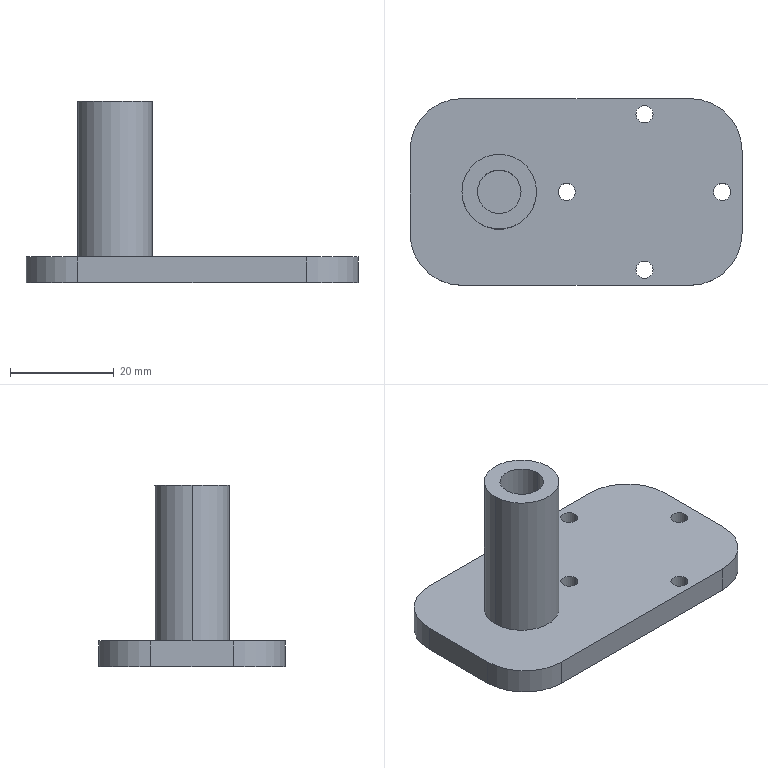Part | SolidWorks | features MirrorStock 1 | 1 solid | 24 faces | box 64 x 36 x 35 mm | volume 14420 mm3 | cylinder 16 | plane 8 | commonest cylinder face diameters 3.3 x8 20 x4 8.4 x2 14.4 x2
STEP:
#1=CARTESIAN_POINT('',(29.65,15.,-22.5));
#2=VERTEX_POINT('',#1);
#3=CARTESIAN_POINT('',(26.35,15.,-22.5));
#4=VERTEX_POINT('',#3);
#5=CARTESIAN_POINT('',(28.,15.,-22.5));
#6=DIRECTION('',(0.,0.,1.));
#7=DIRECTION('',(1.,0.,0.));
#8=AXIS2_PLACEMENT_3D('',#5,#6,#7);
#9=CIRCLE('',#8,1.65);
#10=EDGE_CURVE('',#2,#4,#9,.T.);
#11=ORIENTED_EDGE('',*,*,#10,.T.);
#12=CARTESIAN_POINT('',(26.35,15.,-27.5));
#13=VERTEX_POINT('',#12);
#14=CARTESIAN_POINT('',(26.35,15.,22.5));
#15=DIRECTION('',(0.,0.,-1.));
#16=VECTOR('',#15,1000.);
#17=LINE('',#14,#16);
#18=EDGE_CURVE('',#4,#13,#17,.T.);
#19=ORIENTED_EDGE('',*,*,#18,.T.);
#20=CARTESIAN_POINT('',(29.65,15.,-27.5));
#21=VERTEX_POINT('',#20);
#22=CARTESIAN_POINT('',(28.,15.,-27.5));
#23=DIRECTION('',(0.,0.,1.));
#24=DIRECTION('',(1.,0.,0.));
#25=AXIS2_PLACEMENT_3D('',#22,#23,#24);
#26=CIRCLE('',#25,1.65);
#27=EDGE_CURVE('',#21,#13,#26,.T.);
#28=ORIENTED_EDGE('',*,*,#27,.F.);
#29=CARTESIAN_POINT('',(29.65,15.,22.5));
#30=DIRECTION('',(0.,0.,-1.));
#31=VECTOR('',#30,1000.);
#32=LINE('',#29,#31);
#33=EDGE_CURVE('',#2,#21,#32,.T.);
#34=ORIENTED_EDGE('',*,*,#33,.F.);
#35=EDGE_LOOP('',(#11,#19,#28,#34));
#36=FACE_OUTER_BOUND('',#35,.T.);
#37=CARTESIAN_POINT('',(28.,15.,22.5));
#38=DIRECTION('',(0.,0.,-1.));
#39=DIRECTION('',(1.,0.,0.));
#40=AXIS2_PLACEMENT_3D('',#37,#38,#39);
#41=CYLINDRICAL_SURFACE('',#40,1.65);
#42=ADVANCED_FACE('',(#36),#41,.F.);
#43=CARTESIAN_POINT('',(44.65,0.,-22.5));
#44=VERTEX_POINT('',#43);
#45=CARTESIAN_POINT('',(41.35,0.,-22.5));
#46=VERTEX_POINT('',#45);
#47=CARTESIAN_POINT('',(43.,0.,-22.5));
#48=DIRECTION('',(0.,0.,1.));
#49=DIRECTION('',(1.,0.,0.));
#50=AXIS2_PLACEMENT_3D('',#47,#48,#49);
#51=CIRCLE('',#50,1.65);
#52=EDGE_CURVE('',#44,#46,#51,.T.);
#53=ORIENTED_EDGE('',*,*,#52,.T.);
#54=CARTESIAN_POINT('',(41.35,0.,-27.5));
#55=VERTEX_POINT('',#54);
#56=CARTESIAN_POINT('',(41.35,0.,22.5));
#57=DIRECTION('',(0.,0.,-1.));
#58=VECTOR('',#57,1000.);
#59=LINE('',#56,#58);
#60=EDGE_CURVE('',#46,#55,#59,.T.);
#61=ORIENTED_EDGE('',*,*,#60,.T.);
#62=CARTESIAN_POINT('',(44.65,0.,-27.5));
#63=VERTEX_POINT('',#62);
#64=CARTESIAN_POINT('',(43.,0.,-27.5));
#65=DIRECTION('',(0.,0.,1.));
#66=DIRECTION('',(1.,0.,0.));
#67=AXIS2_PLACEMENT_3D('',#64,#65,#66);
#68=CIRCLE('',#67,1.65);
#69=EDGE_CURVE('',#63,#55,#68,.T.);
#70=ORIENTED_EDGE('',*,*,#69,.F.);
#71=CARTESIAN_POINT('',(44.65,0.,22.5));
#72=DIRECTION('',(0.,0.,-1.));
#73=VECTOR('',#72,1000.);
#74=LINE('',#71,#73);
#75=EDGE_CURVE('',#44,#63,#74,.T.);
#76=ORIENTED_EDGE('',*,*,#75,.F.);
#77=EDGE_LOOP('',(#53,#61,#70,#76));
#78=FACE_OUTER_BOUND('',#77,.T.);
#79=CARTESIAN_POINT('',(43.,0.,22.5));
#80=DIRECTION('',(0.,0.,-1.));
#81=DIRECTION('',(1.,0.,0.));
#82=AXIS2_PLACEMENT_3D('',#79,#80,#81);
#83=CYLINDRICAL_SURFACE('',#82,1.65);
#84=ADVANCED_FACE('',(#78),#83,.F.);
#85=CARTESIAN_POINT('',(29.65,-15.,-22.5));
#86=VERTEX_POINT('',#85);
#87=CARTESIAN_POINT('',(26.35,-15.,-22.5));
#88=VERTEX_POINT('',#87);
#89=CARTESIAN_POINT('',(28.,-15.,-22.5));
#90=DIRECTION('',(0.,0.,1.));
#91=DIRECTION('',(1.,0.,0.));
#92=AXIS2_PLACEMENT_3D('',#89,#90,#91);
#93=CIRCLE('',#92,1.65);
#94=EDGE_CURVE('',#86,#88,#93,.T.);
#95=ORIENTED_EDGE('',*,*,#94,.T.);
#96=CARTESIAN_POINT('',(26.35,-15.,-27.5));
#97=VERTEX_POINT('',#96);
#98=CARTESIAN_POINT('',(26.35,-15.,22.5));
#99=DIRECTION('',(0.,0.,-1.));
#100=VECTOR('',#99,1000.);
#101=LINE('',#98,#100);
#102=EDGE_CURVE('',#88,#97,#101,.T.);
#103=ORIENTED_EDGE('',*,*,#102,.T.);
#104=CARTESIAN_POINT('',(29.65,-15.,-27.5));
#105=VERTEX_POINT('',#104);
#106=CARTESIAN_POINT('',(28.,-15.,-27.5));
#107=DIRECTION('',(0.,0.,1.));
#108=DIRECTION('',(1.,0.,0.));
#109=AXIS2_PLACEMENT_3D('',#106,#107,#108);
#110=CIRCLE('',#109,1.65);
#111=EDGE_CURVE('',#105,#97,#110,.T.);
#112=ORIENTED_EDGE('',*,*,#111,.F.);
#113=CARTESIAN_POINT('',(29.65,-15.,22.5));
#114=DIRECTION('',(0.,0.,-1.));
#115=VECTOR('',#114,1000.);
#116=LINE('',#113,#115);
#117=EDGE_CURVE('',#86,#105,#116,.T.);
#118=ORIENTED_EDGE('',*,*,#117,.F.);
#119=EDGE_LOOP('',(#95,#103,#112,#118));
#120=FACE_OUTER_BOUND('',#119,.T.);
#121=CARTESIAN_POINT('',(28.,-15.,22.5));
#122=DIRECTION('',(0.,0.,-1.));
#123=DIRECTION('',(1.,0.,0.));
#124=AXIS2_PLACEMENT_3D('',#121,#122,#123);
#125=CYLINDRICAL_SURFACE('',#124,1.65);
#126=ADVANCED_FACE('',(#120),#125,.F.);
#127=CARTESIAN_POINT('',(14.65,0.,-22.5));
#128=VERTEX_POINT('',#127);
#129=CARTESIAN_POINT('',(11.35,0.,-22.5));
#130=VERTEX_POINT('',#129);
#131=CARTESIAN_POINT('',(13.,0.,-22.5));
#132=DIRECTION('',(0.,0.,1.));
#133=DIRECTION('',(1.,0.,0.));
#134=AXIS2_PLACEMENT_3D('',#131,#132,#133);
#135=CIRCLE('',#134,1.65);
#136=EDGE_CURVE('',#128,#130,#135,.T.);
#137=ORIENTED_EDGE('',*,*,#136,.T.);
#138=CARTESIAN_POINT('',(11.35,0.,-27.5));
#139=VERTEX_POINT('',#138);
#140=CARTESIAN_POINT('',(11.35,0.,22.5));
#141=DIRECTION('',(0.,0.,-1.));
#142=VECTOR('',#141,1000.);
#143=LINE('',#140,#142);
#144=EDGE_CURVE('',#130,#139,#143,.T.);
#145=ORIENTED_EDGE('',*,*,#144,.T.);
#146=CARTESIAN_POINT('',(14.65,0.,-27.5));
#147=VERTEX_POINT('',#146);
#148=CARTESIAN_POINT('',(13.,0.,-27.5));
#149=DIRECTION('',(0.,0.,1.));
#150=DIRECTION('',(1.,0.,0.));
#151=AXIS2_PLACEMENT_3D('',#148,#149,#150);
#152=CIRCLE('',#151,1.65);
#153=EDGE_CURVE('',#147,#139,#152,.T.);
#154=ORIENTED_EDGE('',*,*,#153,.F.);
#155=CARTESIAN_POINT('',(14.65,0.,22.5));
#156=DIRECTION('',(0.,0.,-1.));
#157=VECTOR('',#156,1000.);
#158=LINE('',#155,#157);
#159=EDGE_CURVE('',#128,#147,#158,.T.);
#160=ORIENTED_EDGE('',*,*,#159,.F.);
#161=EDGE_LOOP('',(#137,#145,#154,#160));
#162=FACE_OUTER_BOUND('',#161,.T.);
#163=CARTESIAN_POINT('',(13.,0.,22.5));
#164=DIRECTION('',(0.,0.,-1.));
#165=DIRECTION('',(1.,0.,0.));
#166=AXIS2_PLACEMENT_3D('',#163,#164,#165);
#167=CYLINDRICAL_SURFACE('',#166,1.65);
#168=ADVANCED_FACE('',(#162),#167,.F.);
#169=CARTESIAN_POINT('',(-4.2,0.,-17.5));
#170=VERTEX_POINT('',#169);
#171=CARTESIAN_POINT('',(4.2,0.,-17.5));
#172=VERTEX_POINT('',#171);
#173=CARTESIAN_POINT('',(0.,0.,-17.5));
#174=DIRECTION('',(0.,0.,-1.));
#175=DIRECTION('',(-1.,0.,0.));
#176=AXIS2_PLACEMENT_3D('',#173,#174,#175);
#177=CIRCLE('',#176,4.2);
#178=EDGE_CURVE('',#170,#172,#177,.T.);
#179=ORIENTED_EDGE('',*,*,#178,.T.);
#180=CARTESIAN_POINT('',(4.2,0.,7.5));
#181=VERTEX_POINT('',#180);
#182=CARTESIAN_POINT('',(4.2,0.,-7.5));
#183=DIRECTION('',(0.,0.,1.));
#184=VECTOR('',#183,1000.);
#185=LINE('',#182,#184);
#186=EDGE_CURVE('',#172,#181,#185,.T.);
#187=ORIENTED_EDGE('',*,*,#186,.T.);
#188=CARTESIAN_POINT('',(-4.2,0.,7.5));
#189=VERTEX_POINT('',#188);
#190=CARTESIAN_POINT('',(0.,0.,7.5));
#191=DIRECTION('',(0.,0.,1.));
#192=DIRECTION('',(1.,0.,0.));
#193=AXIS2_PLACEMENT_3D('',#190,#191,#192);
#194=CIRCLE('',#193,4.2);
#195=EDGE_CURVE('',#181,#189,#194,.T.);
#196=ORIENTED_EDGE('',*,*,#195,.T.);
#197=CARTESIAN_POINT('',(-4.2,0.,-7.5));
#198=DIRECTION('',(0.,0.,1.));
#199=VECTOR('',#198,1000.);
#200=LINE('',#197,#199);
#201=EDGE_CURVE('',#170,#189,#200,.T.);
#202=ORIENTED_EDGE('',*,*,#201,.F.);
#203=EDGE_LOOP('',(#179,#187,#196,#202));
#204=FACE_OUTER_BOUND('',#203,.T.);
#205=CARTESIAN_POINT('',(0.,0.,-7.5));
#206=DIRECTION('',(0.,0.,1.));
#207=DIRECTION('',(-1.,0.,0.));
#208=AXIS2_PLACEMENT_3D('',#205,#206,#207);
#209=CYLINDRICAL_SURFACE('',#208,4.2);
#210=ADVANCED_FACE('',(#204),#209,.F.);
#211=CARTESIAN_POINT('',(-7.2,0.,-22.5));
#212=VERTEX_POINT('',#211);
#213=CARTESIAN_POINT('',(7.2,0.,-22.5));
#214=VERTEX_POINT('',#213);
#215=CARTESIAN_POINT('',(0.,0.,-22.5));
#216=DIRECTION('',(0.,0.,1.));
#217=DIRECTION('',(1.,0.,0.));
#218=AXIS2_PLACEMENT_3D('',#215,#216,#217);
#219=CIRCLE('',#218,7.2);
#220=EDGE_CURVE('',#212,#214,#219,.T.);
#221=ORIENTED_EDGE('',*,*,#220,.T.);
#222=CARTESIAN_POINT('',(7.2,0.,7.5));
#223=VERTEX_POINT('',#222);
#224=CARTESIAN_POINT('',(7.2,0.,-7.5));
#225=DIRECTION('',(0.,0.,1.));
#226=VECTOR('',#225,1000.);
#227=LINE('',#224,#226);
#228=EDGE_CURVE('',#214,#223,#227,.T.);
#229=ORIENTED_EDGE('',*,*,#228,.T.);
#230=CARTESIAN_POINT('',(-7.2,0.,7.5));
#231=VERTEX_POINT('',#230);
#232=CARTESIAN_POINT('',(0.,0.,7.5));
#233=DIRECTION('',(0.,0.,1.));
#234=DIRECTION('',(1.,0.,0.));
#235=AXIS2_PLACEMENT_3D('',#232,#233,#234);
#236=CIRCLE('',#235,7.2);
#237=EDGE_CURVE('',#231,#223,#236,.T.);
#238=ORIENTED_EDGE('',*,*,#237,.F.);
#239=CARTESIAN_POINT('',(-7.2,0.,-7.5));
#240=DIRECTION('',(0.,0.,1.));
#241=VECTOR('',#240,1000.);
#242=LINE('',#239,#241);
#243=EDGE_CURVE('',#212,#231,#242,.T.);
#244=ORIENTED_EDGE('',*,*,#243,.F.);
#245=EDGE_LOOP('',(#221,#229,#238,#244));
#246=FACE_OUTER_BOUND('',#245,.T.);
#247=CARTESIAN_POINT('',(0.,0.,-7.5));
#248=DIRECTION('',(0.,0.,1.));
#249=DIRECTION('',(-1.,0.,0.));
#250=AXIS2_PLACEMENT_3D('',#247,#248,#249);
#251=CYLINDRICAL_SURFACE('',#250,7.2);
#252=ADVANCED_FACE('',(#246),#251,.T.);
#253=ORIENTED_EDGE('',*,*,#228,.F.);
#254=CARTESIAN_POINT('',(0.,0.,-22.5));
#255=DIRECTION('',(0.,0.,1.));
#256=DIRECTION('',(1.,0.,0.));
#257=AXIS2_PLACEMENT_3D('',#254,#255,#256);
#258=CIRCLE('',#257,7.2);
#259=EDGE_CURVE('',#214,#212,#258,.T.);
#260=ORIENTED_EDGE('',*,*,#259,.T.);
#261=ORIENTED_EDGE('',*,*,#243,.T.);
#262=CARTESIAN_POINT('',(0.,0.,7.5));
#263=DIRECTION('',(0.,0.,1.));
#264=DIRECTION('',(1.,0.,0.));
#265=AXIS2_PLACEMENT_3D('',#262,#263,#264);
#266=CIRCLE('',#265,7.2);
#267=EDGE_CURVE('',#223,#231,#266,.T.);
#268=ORIENTED_EDGE('',*,*,#267,.F.);
#269=EDGE_LOOP('',(#253,#260,#261,#268));
#270=FACE_OUTER_BOUND('',#269,.T.);
#271=CARTESIAN_POINT('',(0.,0.,-7.5));
#272=DIRECTION('',(0.,0.,1.));
#273=DIRECTION('',(-1.,0.,0.));
#274=AXIS2_PLACEMENT_3D('',#271,#272,#273);
#275=CYLINDRICAL_SURFACE('',#274,7.2);
#276=ADVANCED_FACE('',(#270),#275,.T.);
#277=ORIENTED_EDGE('',*,*,#186,.F.);
#278=CARTESIAN_POINT('',(0.,0.,-17.5));
#279=DIRECTION('',(0.,0.,-1.));
#280=DIRECTION('',(-1.,0.,0.));
#281=AXIS2_PLACEMENT_3D('',#278,#279,#280);
#282=CIRCLE('',#281,4.2);
#283=EDGE_CURVE('',#172,#170,#282,.T.);
#284=ORIENTED_EDGE('',*,*,#283,.T.);
#285=ORIENTED_EDGE('',*,*,#201,.T.);
#286=CARTESIAN_POINT('',(0.,0.,7.5));
#287=DIRECTION('',(0.,0.,1.));
#288=DIRECTION('',(1.,0.,0.));
#289=AXIS2_PLACEMENT_3D('',#286,#287,#288);
#290=CIRCLE('',#289,4.2);
#291=EDGE_CURVE('',#189,#181,#290,.T.);
#292=ORIENTED_EDGE('',*,*,#291,.T.);
#293=EDGE_LOOP('',(#277,#284,#285,#292));
#294=FACE_OUTER_BOUND('',#293,.T.);
#295=CARTESIAN_POINT('',(0.,0.,-7.5));
#296=DIRECTION('',(0.,0.,1.));
#297=DIRECTION('',(-1.,0.,0.));
#298=AXIS2_PLACEMENT_3D('',#295,#296,#297);
#299=CYLINDRICAL_SURFACE('',#298,4.2);
#300=ADVANCED_FACE('',(#294),#299,.F.);
#301=ORIENTED_EDGE('',*,*,#291,.F.);
#302=ORIENTED_EDGE('',*,*,#195,.F.);
#303=EDGE_LOOP('',(#301,#302));
#304=FACE_BOUND('',#303,.T.);
#305=ORIENTED_EDGE('',*,*,#237,.T.);
#306=ORIENTED_EDGE('',*,*,#267,.T.);
#307=EDGE_LOOP('',(#305,#306));
#308=FACE_OUTER_BOUND('',#307,.T.);
#309=CARTESIAN_POINT('',(0.,0.,7.5));
#310=DIRECTION('',(0.,0.,-1.));
#311=DIRECTION('',(1.,0.,0.));
#312=AXIS2_PLACEMENT_3D('',#309,#310,#311);
#313=PLANE('',#312);
#314=ADVANCED_FACE('',(#304,#308),#313,.F.);
#315=CARTESIAN_POINT('',(-17.2,8.,-27.5));
#316=VERTEX_POINT('',#315);
#317=CARTESIAN_POINT('',(-17.2,-8.,-27.5));
#318=VERTEX_POINT('',#317);
#319=CARTESIAN_POINT('',(-17.2,-18.,-27.5));
#320=DIRECTION('',(0.,-1.,0.));
#321=VECTOR('',#320,1000.);
#322=LINE('',#319,#321);
#323=EDGE_CURVE('',#316,#318,#322,.T.);
#324=ORIENTED_EDGE('',*,*,#323,.T.);
#325=CARTESIAN_POINT('',(-17.2,-8.,-22.5));
#326=VERTEX_POINT('',#325);
#327=CARTESIAN_POINT('',(-17.2,-8.,-22.5));
#328=DIRECTION('',(0.,0.,-1.));
#329=VECTOR('',#328,1000.);
#330=LINE('',#327,#329);
#331=EDGE_CURVE('',#326,#318,#330,.T.);
#332=ORIENTED_EDGE('',*,*,#331,.F.);
#333=CARTESIAN_POINT('',(-17.2,8.,-22.5));
#334=VERTEX_POINT('',#333);
#335=CARTESIAN_POINT('',(-17.2,-18.,-22.5));
#336=DIRECTION('',(0.,-1.,0.));
#337=VECTOR('',#336,1000.);
#338=LINE('',#335,#337);
#339=EDGE_CURVE('',#334,#326,#338,.T.);
#340=ORIENTED_EDGE('',*,*,#339,.F.);
#341=CARTESIAN_POINT('',(-17.2,8.,-22.5));
#342=DIRECTION('',(0.,0.,1.));
#343=VECTOR('',#342,1000.);
#344=LINE('',#341,#343);
#345=EDGE_CURVE('',#316,#334,#344,.T.);
#346=ORIENTED_EDGE('',*,*,#345,.F.);
#347=EDGE_LOOP('',(#324,#332,#340,#346));
#348=FACE_OUTER_BOUND('',#347,.T.);
#349=CARTESIAN_POINT('',(-17.2,-18.,-22.5));
#350=DIRECTION('',(-1.,0.,0.));
#351=DIRECTION('',(0.,0.,-1.));
#352=AXIS2_PLACEMENT_3D('',#349,#350,#351);
#353=PLANE('',#352);
#354=ADVANCED_FACE('',(#348),#353,.T.);
#355=CARTESIAN_POINT('',(36.8,18.,-22.5));
#356=VERTEX_POINT('',#355);
#357=CARTESIAN_POINT('',(-7.2,18.,-22.5));
#358=VERTEX_POINT('',#357);
#359=CARTESIAN_POINT('',(46.8,18.,-22.5));
#360=DIRECTION('',(-1.,0.,0.));
#361=VECTOR('',#360,1000.);
#362=LINE('',#359,#361);
#363=EDGE_CURVE('',#356,#358,#362,.T.);
#364=ORIENTED_EDGE('',*,*,#363,.F.);
#365=CARTESIAN_POINT('',(36.8,18.,-27.5));
#366=VERTEX_POINT('',#365);
#367=CARTESIAN_POINT('',(36.8,18.,-22.5));
#368=DIRECTION('',(0.,0.,1.));
#369=VECTOR('',#368,1000.);
#370=LINE('',#367,#369);
#371=EDGE_CURVE('',#366,#356,#370,.T.);
#372=ORIENTED_EDGE('',*,*,#371,.F.);
#373=CARTESIAN_POINT('',(-7.2,18.,-27.5));
#374=VERTEX_POINT('',#373);
#375=CARTESIAN_POINT('',(46.8,18.,-27.5));
#376=DIRECTION('',(-1.,0.,0.));
#377=VECTOR('',#376,1000.);
#378=LINE('',#375,#377);
#379=EDGE_CURVE('',#366,#374,#378,.T.);
#380=ORIENTED_EDGE('',*,*,#379,.T.);
#381=CARTESIAN_POINT('',(-7.2,18.,-22.5));
#382=DIRECTION('',(0.,0.,-1.));
#383=VECTOR('',#382,1000.);
#384=LINE('',#381,#383);
#385=EDGE_CURVE('',#358,#374,#384,.T.);
#386=ORIENTED_EDGE('',*,*,#385,.F.);
#387=EDGE_LOOP('',(#364,#372,#380,#386));
#388=FACE_OUTER_BOUND('',#387,.T.);
#389=CARTESIAN_POINT('',(46.8,18.,-22.5));
#390=DIRECTION('',(0.,1.,0.));
#391=DIRECTION('',(-1.,0.,0.));
#392=AXIS2_PLACEMENT_3D('',#389,#390,#391);
#393=PLANE('',#392);
#394=ADVANCED_FACE('',(#388),#393,.T.);
#395=CARTESIAN_POINT('',(46.8,-8.,-27.5));
#396=VERTEX_POINT('',#395);
#397=CARTESIAN_POINT('',(46.8,8.,-27.5));
#398=VERTEX_POINT('',#397);
#399=CARTESIAN_POINT('',(46.8,-18.,-27.5));
#400=DIRECTION('',(0.,1.,0.));
#401=VECTOR('',#400,1000.);
#402=LINE('',#399,#401);
#403=EDGE_CURVE('',#396,#398,#402,.T.);
#404=ORIENTED_EDGE('',*,*,#403,.T.);
#405=CARTESIAN_POINT('',(46.8,8.,-22.5));
#406=VERTEX_POINT('',#405);
#407=CARTESIAN_POINT('',(46.8,8.,-22.5));
#408=DIRECTION('',(0.,0.,-1.));
#409=VECTOR('',#408,1000.);
#410=LINE('',#407,#409);
#411=EDGE_CURVE('',#406,#398,#410,.T.);
#412=ORIENTED_EDGE('',*,*,#411,.F.);
#413=CARTESIAN_POINT('',(46.8,-8.,-22.5));
#414=VERTEX_POINT('',#413);
#415=CARTESIAN_POINT('',(46.8,-18.,-22.5));
#416=DIRECTION('',(0.,1.,0.));
#417=VECTOR('',#416,1000.);
#418=LINE('',#415,#417);
#419=EDGE_CURVE('',#414,#406,#418,.T.);
#420=ORIENTED_EDGE('',*,*,#419,.F.);
#421=CARTESIAN_POINT('',(46.8,-8.,-22.5));
#422=DIRECTION('',(0.,0.,1.));
#423=VECTOR('',#422,1000.);
#424=LINE('',#421,#423);
#425=EDGE_CURVE('',#396,#414,#424,.T.);
#426=ORIENTED_EDGE('',*,*,#425,.F.);
#427=EDGE_LOOP('',(#404,#412,#420,#426));
#428=FACE_OUTER_BOUND('',#427,.T.);
#429=CARTESIAN_POINT('',(46.8,-18.,-22.5));
#430=DIRECTION('',(1.,0.,0.));
#431=DIRECTION('',(0.,0.,1.));
#432=AXIS2_PLACEMENT_3D('',#429,#430,#431);
#433=PLANE('',#432);
#434=ADVANCED_FACE('',(#428),#433,.T.);
#435=CARTESIAN_POINT('',(-7.2,-18.,-27.5));
#436=VERTEX_POINT('',#435);
#437=CARTESIAN_POINT('',(36.8,-18.,-27.5));
#438=VERTEX_POINT('',#437);
#439=CARTESIAN_POINT('',(46.8,-18.,-27.5));
#440=DIRECTION('',(1.,0.,0.));
#441=VECTOR('',#440,1000.);
#442=LINE('',#439,#441);
#443=EDGE_CURVE('',#436,#438,#442,.T.);
#444=ORIENTED_EDGE('',*,*,#443,.T.);
#445=CARTESIAN_POINT('',(36.8,-18.,-22.5));
#446=VERTEX_POINT('',#445);
#447=CARTESIAN_POINT('',(36.8,-18.,-22.5));
#448=DIRECTION('',(0.,0.,-1.));
#449=VECTOR('',#448,1000.);
#450=LINE('',#447,#449);
#451=EDGE_CURVE('',#446,#438,#450,.T.);
#452=ORIENTED_EDGE('',*,*,#451,.F.);
#453=CARTESIAN_POINT('',(-7.2,-18.,-22.5));
#454=VERTEX_POINT('',#453);
#455=CARTESIAN_POINT('',(46.8,-18.,-22.5));
#456=DIRECTION('',(1.,0.,0.));
#457=VECTOR('',#456,1000.);
#458=LINE('',#455,#457);
#459=EDGE_CURVE('',#454,#446,#458,.T.);
#460=ORIENTED_EDGE('',*,*,#459,.F.);
#461=CARTESIAN_POINT('',(-7.2,-18.,-22.5));
#462=DIRECTION('',(0.,0.,1.));
#463=VECTOR('',#462,1000.);
#464=LINE('',#461,#463);
#465=EDGE_CURVE('',#436,#454,#464,.T.);
#466=ORIENTED_EDGE('',*,*,#465,.F.);
#467=EDGE_LOOP('',(#444,#452,#460,#466));
#468=FACE_OUTER_BOUND('',#467,.T.);
#469=CARTESIAN_POINT('',(46.8,-18.,-22.5));
#470=DIRECTION('',(0.,-1.,0.));
#471=DIRECTION('',(1.,0.,0.));
#472=AXIS2_PLACEMENT_3D('',#469,#470,#471);
#473=PLANE('',#472);
#474=ADVANCED_FACE('',(#468),#473,.T.);
#475=ORIENTED_EDGE('',*,*,#10,.F.);
#476=CARTESIAN_POINT('',(28.,15.,-22.5));
#477=DIRECTION('',(0.,0.,1.));
#478=DIRECTION('',(1.,0.,0.));
#479=AXIS2_PLACEMENT_3D('',#476,#477,#478);
#480=CIRCLE('',#479,1.65);
#481=EDGE_CURVE('',#4,#2,#480,.T.);
#482=ORIENTED_EDGE('',*,*,#481,.F.);
#483=EDGE_LOOP('',(#475,#482));
#484=FACE_BOUND('',#483,.T.);
#485=ORIENTED_EDGE('',*,*,#52,.F.);
#486=CARTESIAN_POINT('',(43.,0.,-22.5));
#487=DIRECTION('',(0.,0.,1.));
#488=DIRECTION('',(1.,0.,0.));
#489=AXIS2_PLACEMENT_3D('',#486,#487,#488);
#490=CIRCLE('',#489,1.65);
#491=EDGE_CURVE('',#46,#44,#490,.T.);
#492=ORIENTED_EDGE('',*,*,#491,.F.);
#493=EDGE_LOOP('',(#485,#492));
#494=FACE_BOUND('',#493,.T.);
#495=ORIENTED_EDGE('',*,*,#94,.F.);
#496=CARTESIAN_POINT('',(28.,-15.,-22.5));
#497=DIRECTION('',(0.,0.,1.));
#498=DIRECTION('',(1.,0.,0.));
#499=AXIS2_PLACEMENT_3D('',#496,#497,#498);
#500=CIRCLE('',#499,1.65);
#501=EDGE_CURVE('',#88,#86,#500,.T.);
#502=ORIENTED_EDGE('',*,*,#501,.F.);
#503=EDGE_LOOP('',(#495,#502));
#504=FACE_BOUND('',#503,.T.);
#505=ORIENTED_EDGE('',*,*,#136,.F.);
#506=CARTESIAN_POINT('',(13.,0.,-22.5));
#507=DIRECTION('',(0.,0.,1.));
#508=DIRECTION('',(1.,0.,0.));
#509=AXIS2_PLACEMENT_3D('',#506,#507,#508);
#510=CIRCLE('',#509,1.65);
#511=EDGE_CURVE('',#130,#128,#510,.T.);
#512=ORIENTED_EDGE('',*,*,#511,.F.);
#513=EDGE_LOOP('',(#505,#512));
#514=FACE_BOUND('',#513,.T.);
#515=ORIENTED_EDGE('',*,*,#220,.F.);
#516=ORIENTED_EDGE('',*,*,#259,.F.);
#517=EDGE_LOOP('',(#515,#516));
#518=FACE_BOUND('',#517,.T.);
#519=ORIENTED_EDGE('',*,*,#339,.T.);
#520=CARTESIAN_POINT('',(-7.2,-8.,-22.5));
#521=DIRECTION('',(0.,0.,-1.));
#522=DIRECTION('',(1.,0.,0.));
#523=AXIS2_PLACEMENT_3D('',#520,#521,#522);
#524=CIRCLE('',#523,10.);
#525=EDGE_CURVE('',#454,#326,#524,.T.);
#526=ORIENTED_EDGE('',*,*,#525,.F.);
#527=ORIENTED_EDGE('',*,*,#459,.T.);
#528=CARTESIAN_POINT('',(36.8,-8.,-22.5));
#529=DIRECTION('',(0.,0.,-1.));
#530=DIRECTION('',(1.,0.,0.));
#531=AXIS2_PLACEMENT_3D('',#528,#529,#530);
#532=CIRCLE('',#531,10.);
#533=EDGE_CURVE('',#414,#446,#532,.T.);
#534=ORIENTED_EDGE('',*,*,#533,.F.);
#535=ORIENTED_EDGE('',*,*,#419,.T.);
#536=CARTESIAN_POINT('',(36.8,8.,-22.5));
#537=DIRECTION('',(0.,0.,-1.));
#538=DIRECTION('',(1.,0.,0.));
#539=AXIS2_PLACEMENT_3D('',#536,#537,#538);
#540=CIRCLE('',#539,10.);
#541=EDGE_CURVE('',#356,#406,#540,.T.);
#542=ORIENTED_EDGE('',*,*,#541,.F.);
#543=ORIENTED_EDGE('',*,*,#363,.T.);
#544=CARTESIAN_POINT('',(-7.2,8.,-22.5));
#545=DIRECTION('',(0.,0.,-1.));
#546=DIRECTION('',(1.,0.,0.));
#547=AXIS2_PLACEMENT_3D('',#544,#545,#546);
#548=CIRCLE('',#547,10.);
#549=EDGE_CURVE('',#334,#358,#548,.T.);
#550=ORIENTED_EDGE('',*,*,#549,.F.);
#551=EDGE_LOOP('',(#519,#526,#527,#534,#535,#542,#543,#550));
#552=FACE_OUTER_BOUND('',#551,.T.);
#553=CARTESIAN_POINT('',(0.,0.,-22.5));
#554=DIRECTION('',(0.,0.,-1.));
#555=DIRECTION('',(1.,0.,0.));
#556=AXIS2_PLACEMENT_3D('',#553,#554,#555);
#557=PLANE('',#556);
#558=ADVANCED_FACE('',(#484,#494,#504,#514,#518,#552),#557,.F.);
#559=ORIENTED_EDGE('',*,*,#27,.T.);
#560=CARTESIAN_POINT('',(28.,15.,-27.5));
#561=DIRECTION('',(0.,0.,1.));
#562=DIRECTION('',(1.,0.,0.));
#563=AXIS2_PLACEMENT_3D('',#560,#561,#562);
#564=CIRCLE('',#563,1.65);
#565=EDGE_CURVE('',#13,#21,#564,.T.);
#566=ORIENTED_EDGE('',*,*,#565,.T.);
#567=EDGE_LOOP('',(#559,#566));
#568=FACE_BOUND('',#567,.T.);
#569=ORIENTED_EDGE('',*,*,#69,.T.);
#570=CARTESIAN_POINT('',(43.,0.,-27.5));
#571=DIRECTION('',(0.,0.,1.));
#572=DIRECTION('',(1.,0.,0.));
#573=AXIS2_PLACEMENT_3D('',#570,#571,#572);
#574=CIRCLE('',#573,1.65);
#575=EDGE_CURVE('',#55,#63,#574,.T.);
#576=ORIENTED_EDGE('',*,*,#575,.T.);
#577=EDGE_LOOP('',(#569,#576));
#578=FACE_BOUND('',#577,.T.);
#579=ORIENTED_EDGE('',*,*,#111,.T.);
#580=CARTESIAN_POINT('',(28.,-15.,-27.5));
#581=DIRECTION('',(0.,0.,1.));
#582=DIRECTION('',(1.,0.,0.));
#583=AXIS2_PLACEMENT_3D('',#580,#581,#582);
#584=CIRCLE('',#583,1.65);
#585=EDGE_CURVE('',#97,#105,#584,.T.);
#586=ORIENTED_EDGE('',*,*,#585,.T.);
#587=EDGE_LOOP('',(#579,#586));
#588=FACE_BOUND('',#587,.T.);
#589=ORIENTED_EDGE('',*,*,#153,.T.);
#590=CARTESIAN_POINT('',(13.,0.,-27.5));
#591=DIRECTION('',(0.,0.,1.));
#592=DIRECTION('',(1.,0.,0.));
#593=AXIS2_PLACEMENT_3D('',#590,#591,#592);
#594=CIRCLE('',#593,1.65);
#595=EDGE_CURVE('',#139,#147,#594,.T.);
#596=ORIENTED_EDGE('',*,*,#595,.T.);
#597=EDGE_LOOP('',(#589,#596));
#598=FACE_BOUND('',#597,.T.);
#599=ORIENTED_EDGE('',*,*,#379,.F.);
#600=CARTESIAN_POINT('',(36.8,8.,-27.5));
#601=DIRECTION('',(0.,0.,1.));
#602=DIRECTION('',(1.,0.,0.));
#603=AXIS2_PLACEMENT_3D('',#600,#601,#602);
#604=CIRCLE('',#603,10.);
#605=EDGE_CURVE('',#398,#366,#604,.T.);
#606=ORIENTED_EDGE('',*,*,#605,.F.);
#607=ORIENTED_EDGE('',*,*,#403,.F.);
#608=CARTESIAN_POINT('',(36.8,-8.,-27.5));
#609=DIRECTION('',(0.,0.,1.));
#610=DIRECTION('',(1.,0.,0.));
#611=AXIS2_PLACEMENT_3D('',#608,#609,#610);
#612=CIRCLE('',#611,10.);
#613=EDGE_CURVE('',#438,#396,#612,.T.);
#614=ORIENTED_EDGE('',*,*,#613,.F.);
#615=ORIENTED_EDGE('',*,*,#443,.F.);
#616=CARTESIAN_POINT('',(-7.2,-8.,-27.5));
#617=DIRECTION('',(0.,0.,1.));
#618=DIRECTION('',(1.,0.,0.));
#619=AXIS2_PLACEMENT_3D('',#616,#617,#618);
#620=CIRCLE('',#619,10.);
#621=EDGE_CURVE('',#318,#436,#620,.T.);
#622=ORIENTED_EDGE('',*,*,#621,.F.);
#623=ORIENTED_EDGE('',*,*,#323,.F.);
#624=CARTESIAN_POINT('',(-7.2,8.,-27.5));
#625=DIRECTION('',(0.,0.,1.));
#626=DIRECTION('',(1.,0.,0.));
#627=AXIS2_PLACEMENT_3D('',#624,#625,#626);
#628=CIRCLE('',#627,10.);
#629=EDGE_CURVE('',#374,#316,#628,.T.);
#630=ORIENTED_EDGE('',*,*,#629,.F.);
#631=EDGE_LOOP('',(#599,#606,#607,#614,#615,#622,#623,#630));
#632=FACE_OUTER_BOUND('',#631,.T.);
#633=CARTESIAN_POINT('',(0.,0.,-27.5));
#634=DIRECTION('',(0.,0.,-1.));
#635=DIRECTION('',(1.,0.,0.));
#636=AXIS2_PLACEMENT_3D('',#633,#634,#635);
#637=PLANE('',#636);
#638=ADVANCED_FACE('',(#568,#578,#588,#598,#632),#637,.T.);
#639=ORIENTED_EDGE('',*,*,#144,.F.);
#640=ORIENTED_EDGE('',*,*,#511,.T.);
#641=ORIENTED_EDGE('',*,*,#159,.T.);
#642=ORIENTED_EDGE('',*,*,#595,.F.);
#643=EDGE_LOOP('',(#639,#640,#641,#642));
#644=FACE_OUTER_BOUND('',#643,.T.);
#645=CARTESIAN_POINT('',(13.,0.,22.5));
#646=DIRECTION('',(0.,0.,-1.));
#647=DIRECTION('',(1.,0.,0.));
#648=AXIS2_PLACEMENT_3D('',#645,#646,#647);
#649=CYLINDRICAL_SURFACE('',#648,1.65);
#650=ADVANCED_FACE('',(#644),#649,.F.);
#651=ORIENTED_EDGE('',*,*,#102,.F.);
#652=ORIENTED_EDGE('',*,*,#501,.T.);
#653=ORIENTED_EDGE('',*,*,#117,.T.);
#654=ORIENTED_EDGE('',*,*,#585,.F.);
#655=EDGE_LOOP('',(#651,#652,#653,#654));
#656=FACE_OUTER_BOUND('',#655,.T.);
#657=CARTESIAN_POINT('',(28.,-15.,22.5));
#658=DIRECTION('',(0.,0.,-1.));
#659=DIRECTION('',(1.,0.,0.));
#660=AXIS2_PLACEMENT_3D('',#657,#658,#659);
#661=CYLINDRICAL_SURFACE('',#660,1.65);
#662=ADVANCED_FACE('',(#656),#661,.F.);
#663=ORIENTED_EDGE('',*,*,#60,.F.);
#664=ORIENTED_EDGE('',*,*,#491,.T.);
#665=ORIENTED_EDGE('',*,*,#75,.T.);
#666=ORIENTED_EDGE('',*,*,#575,.F.);
#667=EDGE_LOOP('',(#663,#664,#665,#666));
#668=FACE_OUTER_BOUND('',#667,.T.);
#669=CARTESIAN_POINT('',(43.,0.,22.5));
#670=DIRECTION('',(0.,0.,-1.));
#671=DIRECTION('',(1.,0.,0.));
#672=AXIS2_PLACEMENT_3D('',#669,#670,#671);
#673=CYLINDRICAL_SURFACE('',#672,1.65);
#674=ADVANCED_FACE('',(#668),#673,.F.);
#675=ORIENTED_EDGE('',*,*,#18,.F.);
#676=ORIENTED_EDGE('',*,*,#481,.T.);
#677=ORIENTED_EDGE('',*,*,#33,.T.);
#678=ORIENTED_EDGE('',*,*,#565,.F.);
#679=EDGE_LOOP('',(#675,#676,#677,#678));
#680=FACE_OUTER_BOUND('',#679,.T.);
#681=CARTESIAN_POINT('',(28.,15.,22.5));
#682=DIRECTION('',(0.,0.,-1.));
#683=DIRECTION('',(1.,0.,0.));
#684=AXIS2_PLACEMENT_3D('',#681,#682,#683);
#685=CYLINDRICAL_SURFACE('',#684,1.65);
#686=ADVANCED_FACE('',(#680),#685,.F.);
#687=ORIENTED_EDGE('',*,*,#549,.T.);
#688=ORIENTED_EDGE('',*,*,#385,.T.);
#689=ORIENTED_EDGE('',*,*,#629,.T.);
#690=ORIENTED_EDGE('',*,*,#345,.T.);
#691=EDGE_LOOP('',(#687,#688,#689,#690));
#692=FACE_OUTER_BOUND('',#691,.T.);
#693=CARTESIAN_POINT('',(-7.2,8.,-22.5));
#694=DIRECTION('',(0.,0.,-1.));
#695=DIRECTION('',(1.,0.,0.));
#696=AXIS2_PLACEMENT_3D('',#693,#694,#695);
#697=CYLINDRICAL_SURFACE('',#696,10.);
#698=ADVANCED_FACE('',(#692),#697,.T.);
#699=ORIENTED_EDGE('',*,*,#525,.T.);
#700=ORIENTED_EDGE('',*,*,#331,.T.);
#701=ORIENTED_EDGE('',*,*,#621,.T.);
#702=ORIENTED_EDGE('',*,*,#465,.T.);
#703=EDGE_LOOP('',(#699,#700,#701,#702));
#704=FACE_OUTER_BOUND('',#703,.T.);
#705=CARTESIAN_POINT('',(-7.2,-8.,-22.5));
#706=DIRECTION('',(0.,0.,-1.));
#707=DIRECTION('',(1.,0.,0.));
#708=AXIS2_PLACEMENT_3D('',#705,#706,#707);
#709=CYLINDRICAL_SURFACE('',#708,10.);
#710=ADVANCED_FACE('',(#704),#709,.T.);
#711=ORIENTED_EDGE('',*,*,#533,.T.);
#712=ORIENTED_EDGE('',*,*,#451,.T.);
#713=ORIENTED_EDGE('',*,*,#613,.T.);
#714=ORIENTED_EDGE('',*,*,#425,.T.);
#715=EDGE_LOOP('',(#711,#712,#713,#714));
#716=FACE_OUTER_BOUND('',#715,.T.);
#717=CARTESIAN_POINT('',(36.8,-8.,-22.5));
#718=DIRECTION('',(0.,0.,-1.));
#719=DIRECTION('',(1.,0.,0.));
#720=AXIS2_PLACEMENT_3D('',#717,#718,#719);
#721=CYLINDRICAL_SURFACE('',#720,10.);
#722=ADVANCED_FACE('',(#716),#721,.T.);
#723=ORIENTED_EDGE('',*,*,#541,.T.);
#724=ORIENTED_EDGE('',*,*,#411,.T.);
#725=ORIENTED_EDGE('',*,*,#605,.T.);
#726=ORIENTED_EDGE('',*,*,#371,.T.);
#727=EDGE_LOOP('',(#723,#724,#725,#726));
#728=FACE_OUTER_BOUND('',#727,.T.);
#729=CARTESIAN_POINT('',(36.8,8.,-22.5));
#730=DIRECTION('',(0.,0.,-1.));
#731=DIRECTION('',(1.,0.,0.));
#732=AXIS2_PLACEMENT_3D('',#729,#730,#731);
#733=CYLINDRICAL_SURFACE('',#732,10.);
#734=ADVANCED_FACE('',(#728),#733,.T.);
#735=ORIENTED_EDGE('',*,*,#178,.F.);
#736=ORIENTED_EDGE('',*,*,#283,.F.);
#737=EDGE_LOOP('',(#735,#736));
#738=FACE_OUTER_BOUND('',#737,.T.);
#739=CARTESIAN_POINT('',(0.,0.,-17.5));
#740=DIRECTION('',(0.,0.,1.));
#741=DIRECTION('',(-1.,0.,0.));
#742=AXIS2_PLACEMENT_3D('',#739,#740,#741);
#743=PLANE('',#742);
#744=ADVANCED_FACE('',(#738),#743,.T.);
#745=CLOSED_SHELL('',(#42,#84,#126,#168,#210,#252,#276,#300,#314,#354,#394,#434,#474,#558,#638,#650,#662,#674,#686,#698,#710,#722,#734,#744));
#746=MANIFOLD_SOLID_BREP('',#745);
#747=CARTESIAN_POINT('',(0.,0.,0.));
#748=DIRECTION('',(0.,0.,1.));
#749=DIRECTION('',(1.,0.,0.));
#750=AXIS2_PLACEMENT_3D('',#747,#748,#749);
#751=(LENGTH_UNIT()NAMED_UNIT(*)SI_UNIT(.MILLI.,.METRE.));
#752=UNCERTAINTY_MEASURE_WITH_UNIT(LENGTH_MEASURE(0.00001),#751,'','');
#753=(NAMED_UNIT(*)PLANE_ANGLE_UNIT()SI_UNIT($,.RADIAN.));
#754=(NAMED_UNIT(*)SI_UNIT($,.STERADIAN.)SOLID_ANGLE_UNIT());
#755=(GEOMETRIC_REPRESENTATION_CONTEXT(3)GLOBAL_UNCERTAINTY_ASSIGNED_CONTEXT((#752))GLOBAL_UNIT_ASSIGNED_CONTEXT((#751,#753,#754))REPRESENTATION_CONTEXT('',''));
#756=ADVANCED_BREP_SHAPE_REPRESENTATION('',(#746,#750),#755);